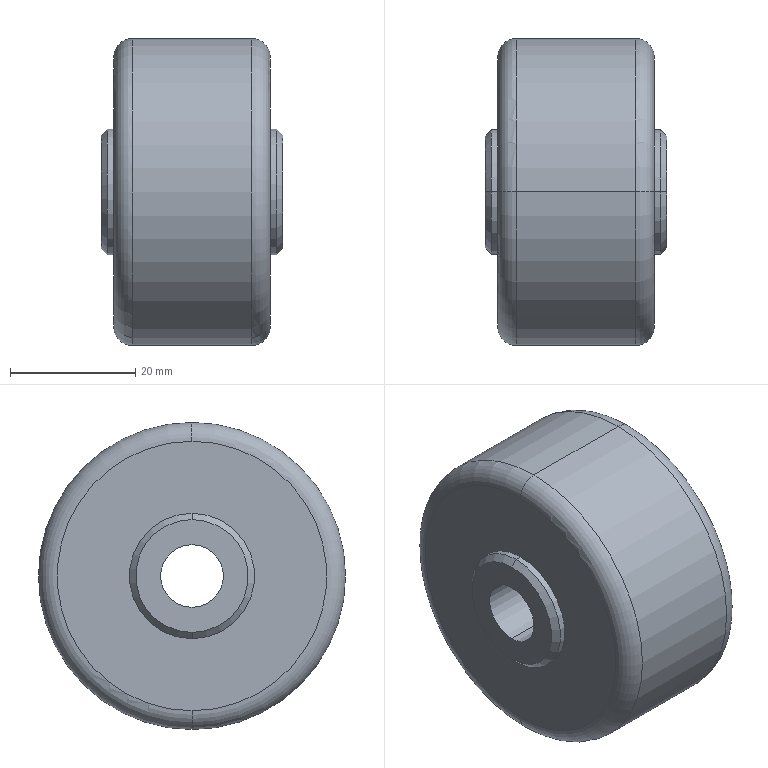Part | STEP file | _CGR51-60-U-001.stp | 1 solid | 20 faces | box 29 x 49 x 49 mm | volume 45483 mm3 | cylinder 8 | cone 4 | torus 4 | plane 4 | commonest cylinder face diameters 20 x4 10 x2 49 x2
STEP:
#1=CARTESIAN_POINT('',(-14.5,0.,-9.));
#2=VERTEX_POINT('',#1);
#3=CARTESIAN_POINT('',(-14.5,0.,9.));
#4=VERTEX_POINT('',#3);
#5=CARTESIAN_POINT('',(-14.5,0.,0.));
#6=DIRECTION('',(1.,0.,0.));
#7=DIRECTION('',(0.,0.,-1.));
#8=AXIS2_PLACEMENT_3D('',#5,#6,#7);
#9=CIRCLE('',#8,9.);
#10=EDGE_CURVE('',#2,#4,#9,.T.);
#11=ORIENTED_EDGE('',*,*,#10,.T.);
#12=CARTESIAN_POINT('',(-13.5,0.,10.));
#13=VERTEX_POINT('',#12);
#14=CARTESIAN_POINT('',(-13.5,0.,10.));
#15=DIRECTION('',(0.7071,0.,0.7071));
#16=VECTOR('',#15,1000.);
#17=LINE('',#14,#16);
#18=EDGE_CURVE('',#4,#13,#17,.T.);
#19=ORIENTED_EDGE('',*,*,#18,.T.);
#20=CARTESIAN_POINT('',(-13.5,0.,-10.));
#21=VERTEX_POINT('',#20);
#22=CARTESIAN_POINT('',(-13.5,0.,0.));
#23=DIRECTION('',(1.,0.,0.));
#24=DIRECTION('',(0.,0.,-1.));
#25=AXIS2_PLACEMENT_3D('',#22,#23,#24);
#26=CIRCLE('',#25,10.);
#27=EDGE_CURVE('',#21,#13,#26,.T.);
#28=ORIENTED_EDGE('',*,*,#27,.F.);
#29=CARTESIAN_POINT('',(-13.5,0.,-10.));
#30=DIRECTION('',(0.7071,0.,-0.7071));
#31=VECTOR('',#30,1000.);
#32=LINE('',#29,#31);
#33=EDGE_CURVE('',#2,#21,#32,.T.);
#34=ORIENTED_EDGE('',*,*,#33,.F.);
#35=EDGE_LOOP('',(#11,#19,#28,#34));
#36=FACE_OUTER_BOUND('',#35,.T.);
#37=CARTESIAN_POINT('',(-13.5,0.,0.));
#38=DIRECTION('',(1.,0.,0.));
#39=DIRECTION('',(0.,0.,-1.));
#40=AXIS2_PLACEMENT_3D('',#37,#38,#39);
#41=CONICAL_SURFACE('',#40,10.,0.7854);
#42=ADVANCED_FACE('',(#36),#41,.T.);
#43=CARTESIAN_POINT('',(14.5,0.,-5.));
#44=VERTEX_POINT('',#43);
#45=CARTESIAN_POINT('',(14.5,0.,5.));
#46=VERTEX_POINT('',#45);
#47=CARTESIAN_POINT('',(14.5,0.,0.));
#48=DIRECTION('',(1.,0.,0.));
#49=DIRECTION('',(0.,0.,-1.));
#50=AXIS2_PLACEMENT_3D('',#47,#48,#49);
#51=CIRCLE('',#50,5.);
#52=EDGE_CURVE('',#44,#46,#51,.T.);
#53=ORIENTED_EDGE('',*,*,#52,.T.);
#54=CARTESIAN_POINT('',(-14.5,0.,5.));
#55=VERTEX_POINT('',#54);
#56=CARTESIAN_POINT('',(50.,0.,5.));
#57=DIRECTION('',(-1.,0.,0.));
#58=VECTOR('',#57,1000.);
#59=LINE('',#56,#58);
#60=EDGE_CURVE('',#46,#55,#59,.T.);
#61=ORIENTED_EDGE('',*,*,#60,.T.);
#62=CARTESIAN_POINT('',(-14.5,0.,-5.));
#63=VERTEX_POINT('',#62);
#64=CARTESIAN_POINT('',(-14.5,0.,0.));
#65=DIRECTION('',(1.,0.,0.));
#66=DIRECTION('',(0.,0.,-1.));
#67=AXIS2_PLACEMENT_3D('',#64,#65,#66);
#68=CIRCLE('',#67,5.);
#69=EDGE_CURVE('',#63,#55,#68,.T.);
#70=ORIENTED_EDGE('',*,*,#69,.F.);
#71=CARTESIAN_POINT('',(50.,0.,-5.));
#72=DIRECTION('',(-1.,0.,0.));
#73=VECTOR('',#72,1000.);
#74=LINE('',#71,#73);
#75=EDGE_CURVE('',#44,#63,#74,.T.);
#76=ORIENTED_EDGE('',*,*,#75,.F.);
#77=EDGE_LOOP('',(#53,#61,#70,#76));
#78=FACE_OUTER_BOUND('',#77,.T.);
#79=CARTESIAN_POINT('',(50.,0.,0.));
#80=DIRECTION('',(-1.,0.,0.));
#81=DIRECTION('',(0.,0.,-1.));
#82=AXIS2_PLACEMENT_3D('',#79,#80,#81);
#83=CYLINDRICAL_SURFACE('',#82,5.);
#84=ADVANCED_FACE('',(#78),#83,.F.);
#85=CARTESIAN_POINT('',(14.5,0.,-9.));
#86=VERTEX_POINT('',#85);
#87=CARTESIAN_POINT('',(14.5,0.,9.));
#88=VERTEX_POINT('',#87);
#89=CARTESIAN_POINT('',(14.5,0.,0.));
#90=DIRECTION('',(1.,0.,0.));
#91=DIRECTION('',(0.,0.,-1.));
#92=AXIS2_PLACEMENT_3D('',#89,#90,#91);
#93=CIRCLE('',#92,9.);
#94=EDGE_CURVE('',#86,#88,#93,.T.);
#95=ORIENTED_EDGE('',*,*,#94,.F.);
#96=CARTESIAN_POINT('',(13.5,0.,-10.));
#97=VERTEX_POINT('',#96);
#98=CARTESIAN_POINT('',(14.5,0.,-9.));
#99=DIRECTION('',(-0.7071,0.,-0.7071));
#100=VECTOR('',#99,1000.);
#101=LINE('',#98,#100);
#102=EDGE_CURVE('',#86,#97,#101,.T.);
#103=ORIENTED_EDGE('',*,*,#102,.T.);
#104=CARTESIAN_POINT('',(13.5,0.,10.));
#105=VERTEX_POINT('',#104);
#106=CARTESIAN_POINT('',(13.5,0.,0.));
#107=DIRECTION('',(1.,0.,0.));
#108=DIRECTION('',(0.,0.,-1.));
#109=AXIS2_PLACEMENT_3D('',#106,#107,#108);
#110=CIRCLE('',#109,10.);
#111=EDGE_CURVE('',#97,#105,#110,.T.);
#112=ORIENTED_EDGE('',*,*,#111,.T.);
#113=CARTESIAN_POINT('',(14.5,0.,9.));
#114=DIRECTION('',(-0.7071,0.,0.7071));
#115=VECTOR('',#114,1000.);
#116=LINE('',#113,#115);
#117=EDGE_CURVE('',#88,#105,#116,.T.);
#118=ORIENTED_EDGE('',*,*,#117,.F.);
#119=EDGE_LOOP('',(#95,#103,#112,#118));
#120=FACE_OUTER_BOUND('',#119,.T.);
#121=CARTESIAN_POINT('',(14.5,0.,0.));
#122=DIRECTION('',(-1.,0.,0.));
#123=DIRECTION('',(0.,0.,1.));
#124=AXIS2_PLACEMENT_3D('',#121,#122,#123);
#125=CONICAL_SURFACE('',#124,9.,0.7854);
#126=ADVANCED_FACE('',(#120),#125,.T.);
#127=CARTESIAN_POINT('',(13.5,0.,0.));
#128=DIRECTION('',(1.,0.,0.));
#129=DIRECTION('',(0.,0.,-1.));
#130=AXIS2_PLACEMENT_3D('',#127,#128,#129);
#131=CIRCLE('',#130,10.);
#132=EDGE_CURVE('',#105,#97,#131,.T.);
#133=ORIENTED_EDGE('',*,*,#132,.F.);
#134=CARTESIAN_POINT('',(12.5,0.,10.));
#135=VERTEX_POINT('',#134);
#136=CARTESIAN_POINT('',(50.,0.,10.));
#137=DIRECTION('',(-1.,0.,0.));
#138=VECTOR('',#137,1000.);
#139=LINE('',#136,#138);
#140=EDGE_CURVE('',#105,#135,#139,.T.);
#141=ORIENTED_EDGE('',*,*,#140,.T.);
#142=CARTESIAN_POINT('',(12.5,0.,-10.));
#143=VERTEX_POINT('',#142);
#144=CARTESIAN_POINT('',(12.5,0.,0.));
#145=DIRECTION('',(1.,0.,0.));
#146=DIRECTION('',(0.,0.,-1.));
#147=AXIS2_PLACEMENT_3D('',#144,#145,#146);
#148=CIRCLE('',#147,10.);
#149=EDGE_CURVE('',#135,#143,#148,.T.);
#150=ORIENTED_EDGE('',*,*,#149,.T.);
#151=CARTESIAN_POINT('',(50.,0.,-10.));
#152=DIRECTION('',(-1.,0.,0.));
#153=VECTOR('',#152,1000.);
#154=LINE('',#151,#153);
#155=EDGE_CURVE('',#97,#143,#154,.T.);
#156=ORIENTED_EDGE('',*,*,#155,.F.);
#157=EDGE_LOOP('',(#133,#141,#150,#156));
#158=FACE_OUTER_BOUND('',#157,.T.);
#159=CARTESIAN_POINT('',(50.,0.,0.));
#160=DIRECTION('',(-1.,0.,0.));
#161=DIRECTION('',(0.,0.,-1.));
#162=AXIS2_PLACEMENT_3D('',#159,#160,#161);
#163=CYLINDRICAL_SURFACE('',#162,10.);
#164=ADVANCED_FACE('',(#158),#163,.T.);
#165=CARTESIAN_POINT('',(9.5,0.,-24.5));
#166=VERTEX_POINT('',#165);
#167=CARTESIAN_POINT('',(9.5,0.,24.5));
#168=VERTEX_POINT('',#167);
#169=CARTESIAN_POINT('',(9.5,0.,0.));
#170=DIRECTION('',(1.,0.,0.));
#171=DIRECTION('',(0.,0.,-1.));
#172=AXIS2_PLACEMENT_3D('',#169,#170,#171);
#173=CIRCLE('',#172,24.5);
#174=EDGE_CURVE('',#166,#168,#173,.T.);
#175=ORIENTED_EDGE('',*,*,#174,.T.);
#176=CARTESIAN_POINT('',(12.5,0.,21.5));
#177=VERTEX_POINT('',#176);
#178=CARTESIAN_POINT('',(9.5,0.,21.5));
#179=DIRECTION('',(0.,1.,0.));
#180=DIRECTION('',(0.,0.,1.));
#181=AXIS2_PLACEMENT_3D('',#178,#179,#180);
#182=CIRCLE('',#181,3.);
#183=EDGE_CURVE('',#168,#177,#182,.T.);
#184=ORIENTED_EDGE('',*,*,#183,.T.);
#185=CARTESIAN_POINT('',(12.5,0.,-21.5));
#186=VERTEX_POINT('',#185);
#187=CARTESIAN_POINT('',(12.5,0.,0.));
#188=DIRECTION('',(1.,0.,0.));
#189=DIRECTION('',(0.,0.,-1.));
#190=AXIS2_PLACEMENT_3D('',#187,#188,#189);
#191=CIRCLE('',#190,21.5);
#192=EDGE_CURVE('',#186,#177,#191,.T.);
#193=ORIENTED_EDGE('',*,*,#192,.F.);
#194=CARTESIAN_POINT('',(9.5,0.,-21.5));
#195=DIRECTION('',(0.,-1.,0.));
#196=DIRECTION('',(0.,0.,-1.));
#197=AXIS2_PLACEMENT_3D('',#194,#195,#196);
#198=CIRCLE('',#197,3.);
#199=EDGE_CURVE('',#166,#186,#198,.T.);
#200=ORIENTED_EDGE('',*,*,#199,.F.);
#201=EDGE_LOOP('',(#175,#184,#193,#200));
#202=FACE_OUTER_BOUND('',#201,.T.);
#203=CARTESIAN_POINT('',(9.5,0.,0.));
#204=DIRECTION('',(1.,0.,0.));
#205=DIRECTION('',(0.,0.,-1.));
#206=AXIS2_PLACEMENT_3D('',#203,#204,#205);
#207=TOROIDAL_SURFACE('',#206,21.5,3.);
#208=ADVANCED_FACE('',(#202),#207,.T.);
#209=CARTESIAN_POINT('',(9.5,0.,0.));
#210=DIRECTION('',(1.,0.,0.));
#211=DIRECTION('',(0.,0.,-1.));
#212=AXIS2_PLACEMENT_3D('',#209,#210,#211);
#213=CIRCLE('',#212,24.5);
#214=EDGE_CURVE('',#168,#166,#213,.T.);
#215=ORIENTED_EDGE('',*,*,#214,.F.);
#216=CARTESIAN_POINT('',(-9.5,0.,24.5));
#217=VERTEX_POINT('',#216);
#218=CARTESIAN_POINT('',(50.,0.,24.5));
#219=DIRECTION('',(-1.,0.,0.));
#220=VECTOR('',#219,1000.);
#221=LINE('',#218,#220);
#222=EDGE_CURVE('',#168,#217,#221,.T.);
#223=ORIENTED_EDGE('',*,*,#222,.T.);
#224=CARTESIAN_POINT('',(-9.5,0.,-24.5));
#225=VERTEX_POINT('',#224);
#226=CARTESIAN_POINT('',(-9.5,0.,0.));
#227=DIRECTION('',(1.,0.,0.));
#228=DIRECTION('',(0.,0.,-1.));
#229=AXIS2_PLACEMENT_3D('',#226,#227,#228);
#230=CIRCLE('',#229,24.5);
#231=EDGE_CURVE('',#217,#225,#230,.T.);
#232=ORIENTED_EDGE('',*,*,#231,.T.);
#233=CARTESIAN_POINT('',(50.,0.,-24.5));
#234=DIRECTION('',(-1.,0.,0.));
#235=VECTOR('',#234,1000.);
#236=LINE('',#233,#235);
#237=EDGE_CURVE('',#166,#225,#236,.T.);
#238=ORIENTED_EDGE('',*,*,#237,.F.);
#239=EDGE_LOOP('',(#215,#223,#232,#238));
#240=FACE_OUTER_BOUND('',#239,.T.);
#241=CARTESIAN_POINT('',(50.,0.,0.));
#242=DIRECTION('',(-1.,0.,0.));
#243=DIRECTION('',(0.,0.,-1.));
#244=AXIS2_PLACEMENT_3D('',#241,#242,#243);
#245=CYLINDRICAL_SURFACE('',#244,24.5);
#246=ADVANCED_FACE('',(#240),#245,.T.);
#247=CARTESIAN_POINT('',(-12.5,0.,-21.5));
#248=VERTEX_POINT('',#247);
#249=CARTESIAN_POINT('',(-12.5,0.,21.5));
#250=VERTEX_POINT('',#249);
#251=CARTESIAN_POINT('',(-12.5,0.,0.));
#252=DIRECTION('',(1.,0.,0.));
#253=DIRECTION('',(0.,0.,-1.));
#254=AXIS2_PLACEMENT_3D('',#251,#252,#253);
#255=CIRCLE('',#254,21.5);
#256=EDGE_CURVE('',#248,#250,#255,.T.);
#257=ORIENTED_EDGE('',*,*,#256,.T.);
#258=CARTESIAN_POINT('',(-9.5,0.,21.5));
#259=DIRECTION('',(0.,1.,0.));
#260=DIRECTION('',(0.,0.,1.));
#261=AXIS2_PLACEMENT_3D('',#258,#259,#260);
#262=CIRCLE('',#261,3.);
#263=EDGE_CURVE('',#250,#217,#262,.T.);
#264=ORIENTED_EDGE('',*,*,#263,.T.);
#265=CARTESIAN_POINT('',(-9.5,0.,0.));
#266=DIRECTION('',(1.,0.,0.));
#267=DIRECTION('',(0.,0.,-1.));
#268=AXIS2_PLACEMENT_3D('',#265,#266,#267);
#269=CIRCLE('',#268,24.5);
#270=EDGE_CURVE('',#225,#217,#269,.T.);
#271=ORIENTED_EDGE('',*,*,#270,.F.);
#272=CARTESIAN_POINT('',(-9.5,0.,-21.5));
#273=DIRECTION('',(0.,-1.,0.));
#274=DIRECTION('',(0.,0.,-1.));
#275=AXIS2_PLACEMENT_3D('',#272,#273,#274);
#276=CIRCLE('',#275,3.);
#277=EDGE_CURVE('',#248,#225,#276,.T.);
#278=ORIENTED_EDGE('',*,*,#277,.F.);
#279=EDGE_LOOP('',(#257,#264,#271,#278));
#280=FACE_OUTER_BOUND('',#279,.T.);
#281=CARTESIAN_POINT('',(-9.5,0.,0.));
#282=DIRECTION('',(1.,0.,0.));
#283=DIRECTION('',(0.,0.,-1.));
#284=AXIS2_PLACEMENT_3D('',#281,#282,#283);
#285=TOROIDAL_SURFACE('',#284,21.5,3.);
#286=ADVANCED_FACE('',(#280),#285,.T.);
#287=CARTESIAN_POINT('',(-12.5,0.,10.));
#288=VERTEX_POINT('',#287);
#289=CARTESIAN_POINT('',(-12.5,0.,-10.));
#290=VERTEX_POINT('',#289);
#291=CARTESIAN_POINT('',(-12.5,0.,0.));
#292=DIRECTION('',(1.,0.,0.));
#293=DIRECTION('',(0.,0.,-1.));
#294=AXIS2_PLACEMENT_3D('',#291,#292,#293);
#295=CIRCLE('',#294,10.);
#296=EDGE_CURVE('',#288,#290,#295,.T.);
#297=ORIENTED_EDGE('',*,*,#296,.F.);
#298=CARTESIAN_POINT('',(50.,0.,10.));
#299=DIRECTION('',(-1.,0.,0.));
#300=VECTOR('',#299,1000.);
#301=LINE('',#298,#300);
#302=EDGE_CURVE('',#288,#13,#301,.T.);
#303=ORIENTED_EDGE('',*,*,#302,.T.);
#304=CARTESIAN_POINT('',(-13.5,0.,0.));
#305=DIRECTION('',(1.,0.,0.));
#306=DIRECTION('',(0.,0.,-1.));
#307=AXIS2_PLACEMENT_3D('',#304,#305,#306);
#308=CIRCLE('',#307,10.);
#309=EDGE_CURVE('',#13,#21,#308,.T.);
#310=ORIENTED_EDGE('',*,*,#309,.T.);
#311=CARTESIAN_POINT('',(50.,0.,-10.));
#312=DIRECTION('',(-1.,0.,0.));
#313=VECTOR('',#312,1000.);
#314=LINE('',#311,#313);
#315=EDGE_CURVE('',#290,#21,#314,.T.);
#316=ORIENTED_EDGE('',*,*,#315,.F.);
#317=EDGE_LOOP('',(#297,#303,#310,#316));
#318=FACE_OUTER_BOUND('',#317,.T.);
#319=CARTESIAN_POINT('',(50.,0.,0.));
#320=DIRECTION('',(-1.,0.,0.));
#321=DIRECTION('',(0.,0.,-1.));
#322=AXIS2_PLACEMENT_3D('',#319,#320,#321);
#323=CYLINDRICAL_SURFACE('',#322,10.);
#324=ADVANCED_FACE('',(#318),#323,.T.);
#325=ORIENTED_EDGE('',*,*,#302,.F.);
#326=CARTESIAN_POINT('',(-12.5,0.,0.));
#327=DIRECTION('',(1.,0.,0.));
#328=DIRECTION('',(0.,0.,-1.));
#329=AXIS2_PLACEMENT_3D('',#326,#327,#328);
#330=CIRCLE('',#329,10.);
#331=EDGE_CURVE('',#290,#288,#330,.T.);
#332=ORIENTED_EDGE('',*,*,#331,.F.);
#333=ORIENTED_EDGE('',*,*,#315,.T.);
#334=ORIENTED_EDGE('',*,*,#27,.T.);
#335=EDGE_LOOP('',(#325,#332,#333,#334));
#336=FACE_OUTER_BOUND('',#335,.T.);
#337=CARTESIAN_POINT('',(50.,0.,0.));
#338=DIRECTION('',(-1.,0.,0.));
#339=DIRECTION('',(0.,0.,-1.));
#340=AXIS2_PLACEMENT_3D('',#337,#338,#339);
#341=CYLINDRICAL_SURFACE('',#340,10.);
#342=ADVANCED_FACE('',(#336),#341,.T.);
#343=ORIENTED_EDGE('',*,*,#331,.T.);
#344=ORIENTED_EDGE('',*,*,#296,.T.);
#345=EDGE_LOOP('',(#343,#344));
#346=FACE_BOUND('',#345,.T.);
#347=ORIENTED_EDGE('',*,*,#256,.F.);
#348=CARTESIAN_POINT('',(-12.5,0.,0.));
#349=DIRECTION('',(1.,0.,0.));
#350=DIRECTION('',(0.,0.,-1.));
#351=AXIS2_PLACEMENT_3D('',#348,#349,#350);
#352=CIRCLE('',#351,21.5);
#353=EDGE_CURVE('',#250,#248,#352,.T.);
#354=ORIENTED_EDGE('',*,*,#353,.F.);
#355=EDGE_LOOP('',(#347,#354));
#356=FACE_OUTER_BOUND('',#355,.T.);
#357=CARTESIAN_POINT('',(-12.5,21.5,0.));
#358=DIRECTION('',(-1.,0.,0.));
#359=DIRECTION('',(0.,0.,1.));
#360=AXIS2_PLACEMENT_3D('',#357,#358,#359);
#361=PLANE('',#360);
#362=ADVANCED_FACE('',(#346,#356),#361,.T.);
#363=ORIENTED_EDGE('',*,*,#263,.F.);
#364=ORIENTED_EDGE('',*,*,#353,.T.);
#365=ORIENTED_EDGE('',*,*,#277,.T.);
#366=ORIENTED_EDGE('',*,*,#231,.F.);
#367=EDGE_LOOP('',(#363,#364,#365,#366));
#368=FACE_OUTER_BOUND('',#367,.T.);
#369=CARTESIAN_POINT('',(-9.5,0.,0.));
#370=DIRECTION('',(1.,0.,0.));
#371=DIRECTION('',(0.,0.,-1.));
#372=AXIS2_PLACEMENT_3D('',#369,#370,#371);
#373=TOROIDAL_SURFACE('',#372,21.5,3.);
#374=ADVANCED_FACE('',(#368),#373,.T.);
#375=ORIENTED_EDGE('',*,*,#222,.F.);
#376=ORIENTED_EDGE('',*,*,#174,.F.);
#377=ORIENTED_EDGE('',*,*,#237,.T.);
#378=ORIENTED_EDGE('',*,*,#270,.T.);
#379=EDGE_LOOP('',(#375,#376,#377,#378));
#380=FACE_OUTER_BOUND('',#379,.T.);
#381=CARTESIAN_POINT('',(50.,0.,0.));
#382=DIRECTION('',(-1.,0.,0.));
#383=DIRECTION('',(0.,0.,-1.));
#384=AXIS2_PLACEMENT_3D('',#381,#382,#383);
#385=CYLINDRICAL_SURFACE('',#384,24.5);
#386=ADVANCED_FACE('',(#380),#385,.T.);
#387=ORIENTED_EDGE('',*,*,#183,.F.);
#388=ORIENTED_EDGE('',*,*,#214,.T.);
#389=ORIENTED_EDGE('',*,*,#199,.T.);
#390=CARTESIAN_POINT('',(12.5,0.,0.));
#391=DIRECTION('',(1.,0.,0.));
#392=DIRECTION('',(0.,0.,-1.));
#393=AXIS2_PLACEMENT_3D('',#390,#391,#392);
#394=CIRCLE('',#393,21.5);
#395=EDGE_CURVE('',#177,#186,#394,.T.);
#396=ORIENTED_EDGE('',*,*,#395,.F.);
#397=EDGE_LOOP('',(#387,#388,#389,#396));
#398=FACE_OUTER_BOUND('',#397,.T.);
#399=CARTESIAN_POINT('',(9.5,0.,0.));
#400=DIRECTION('',(1.,0.,0.));
#401=DIRECTION('',(0.,0.,-1.));
#402=AXIS2_PLACEMENT_3D('',#399,#400,#401);
#403=TOROIDAL_SURFACE('',#402,21.5,3.);
#404=ADVANCED_FACE('',(#398),#403,.T.);
#405=CARTESIAN_POINT('',(12.5,0.,0.));
#406=DIRECTION('',(1.,0.,0.));
#407=DIRECTION('',(0.,0.,-1.));
#408=AXIS2_PLACEMENT_3D('',#405,#406,#407);
#409=CIRCLE('',#408,10.);
#410=EDGE_CURVE('',#143,#135,#409,.T.);
#411=ORIENTED_EDGE('',*,*,#410,.F.);
#412=ORIENTED_EDGE('',*,*,#149,.F.);
#413=EDGE_LOOP('',(#411,#412));
#414=FACE_BOUND('',#413,.T.);
#415=ORIENTED_EDGE('',*,*,#192,.T.);
#416=ORIENTED_EDGE('',*,*,#395,.T.);
#417=EDGE_LOOP('',(#415,#416));
#418=FACE_OUTER_BOUND('',#417,.T.);
#419=CARTESIAN_POINT('',(12.5,10.,0.));
#420=DIRECTION('',(1.,0.,0.));
#421=DIRECTION('',(0.,1.,0.));
#422=AXIS2_PLACEMENT_3D('',#419,#420,#421);
#423=PLANE('',#422);
#424=ADVANCED_FACE('',(#414,#418),#423,.T.);
#425=ORIENTED_EDGE('',*,*,#140,.F.);
#426=ORIENTED_EDGE('',*,*,#111,.F.);
#427=ORIENTED_EDGE('',*,*,#155,.T.);
#428=ORIENTED_EDGE('',*,*,#410,.T.);
#429=EDGE_LOOP('',(#425,#426,#427,#428));
#430=FACE_OUTER_BOUND('',#429,.T.);
#431=CARTESIAN_POINT('',(50.,0.,0.));
#432=DIRECTION('',(-1.,0.,0.));
#433=DIRECTION('',(0.,0.,-1.));
#434=AXIS2_PLACEMENT_3D('',#431,#432,#433);
#435=CYLINDRICAL_SURFACE('',#434,10.);
#436=ADVANCED_FACE('',(#430),#435,.T.);
#437=ORIENTED_EDGE('',*,*,#102,.F.);
#438=CARTESIAN_POINT('',(14.5,0.,0.));
#439=DIRECTION('',(1.,0.,0.));
#440=DIRECTION('',(0.,0.,-1.));
#441=AXIS2_PLACEMENT_3D('',#438,#439,#440);
#442=CIRCLE('',#441,9.);
#443=EDGE_CURVE('',#88,#86,#442,.T.);
#444=ORIENTED_EDGE('',*,*,#443,.F.);
#445=ORIENTED_EDGE('',*,*,#117,.T.);
#446=ORIENTED_EDGE('',*,*,#132,.T.);
#447=EDGE_LOOP('',(#437,#444,#445,#446));
#448=FACE_OUTER_BOUND('',#447,.T.);
#449=CARTESIAN_POINT('',(14.5,0.,0.));
#450=DIRECTION('',(-1.,0.,0.));
#451=DIRECTION('',(0.,0.,1.));
#452=AXIS2_PLACEMENT_3D('',#449,#450,#451);
#453=CONICAL_SURFACE('',#452,9.,0.7854);
#454=ADVANCED_FACE('',(#448),#453,.T.);
#455=ORIENTED_EDGE('',*,*,#52,.F.);
#456=CARTESIAN_POINT('',(14.5,0.,0.));
#457=DIRECTION('',(1.,0.,0.));
#458=DIRECTION('',(0.,0.,-1.));
#459=AXIS2_PLACEMENT_3D('',#456,#457,#458);
#460=CIRCLE('',#459,5.);
#461=EDGE_CURVE('',#46,#44,#460,.T.);
#462=ORIENTED_EDGE('',*,*,#461,.F.);
#463=EDGE_LOOP('',(#455,#462));
#464=FACE_BOUND('',#463,.T.);
#465=ORIENTED_EDGE('',*,*,#443,.T.);
#466=ORIENTED_EDGE('',*,*,#94,.T.);
#467=EDGE_LOOP('',(#465,#466));
#468=FACE_OUTER_BOUND('',#467,.T.);
#469=CARTESIAN_POINT('',(14.5,5.,0.));
#470=DIRECTION('',(1.,0.,0.));
#471=DIRECTION('',(0.,1.,0.));
#472=AXIS2_PLACEMENT_3D('',#469,#470,#471);
#473=PLANE('',#472);
#474=ADVANCED_FACE('',(#464,#468),#473,.T.);
#475=ORIENTED_EDGE('',*,*,#60,.F.);
#476=ORIENTED_EDGE('',*,*,#461,.T.);
#477=ORIENTED_EDGE('',*,*,#75,.T.);
#478=CARTESIAN_POINT('',(-14.5,0.,0.));
#479=DIRECTION('',(1.,0.,0.));
#480=DIRECTION('',(0.,0.,-1.));
#481=AXIS2_PLACEMENT_3D('',#478,#479,#480);
#482=CIRCLE('',#481,5.);
#483=EDGE_CURVE('',#55,#63,#482,.T.);
#484=ORIENTED_EDGE('',*,*,#483,.F.);
#485=EDGE_LOOP('',(#475,#476,#477,#484));
#486=FACE_OUTER_BOUND('',#485,.T.);
#487=CARTESIAN_POINT('',(50.,0.,0.));
#488=DIRECTION('',(-1.,0.,0.));
#489=DIRECTION('',(0.,0.,-1.));
#490=AXIS2_PLACEMENT_3D('',#487,#488,#489);
#491=CYLINDRICAL_SURFACE('',#490,5.);
#492=ADVANCED_FACE('',(#486),#491,.F.);
#493=ORIENTED_EDGE('',*,*,#69,.T.);
#494=ORIENTED_EDGE('',*,*,#483,.T.);
#495=EDGE_LOOP('',(#493,#494));
#496=FACE_BOUND('',#495,.T.);
#497=ORIENTED_EDGE('',*,*,#10,.F.);
#498=CARTESIAN_POINT('',(-14.5,0.,0.));
#499=DIRECTION('',(1.,0.,0.));
#500=DIRECTION('',(0.,0.,-1.));
#501=AXIS2_PLACEMENT_3D('',#498,#499,#500);
#502=CIRCLE('',#501,9.);
#503=EDGE_CURVE('',#4,#2,#502,.T.);
#504=ORIENTED_EDGE('',*,*,#503,.F.);
#505=EDGE_LOOP('',(#497,#504));
#506=FACE_OUTER_BOUND('',#505,.T.);
#507=CARTESIAN_POINT('',(-14.5,9.,0.));
#508=DIRECTION('',(-1.,0.,0.));
#509=DIRECTION('',(0.,0.,1.));
#510=AXIS2_PLACEMENT_3D('',#507,#508,#509);
#511=PLANE('',#510);
#512=ADVANCED_FACE('',(#496,#506),#511,.T.);
#513=ORIENTED_EDGE('',*,*,#18,.F.);
#514=ORIENTED_EDGE('',*,*,#503,.T.);
#515=ORIENTED_EDGE('',*,*,#33,.T.);
#516=ORIENTED_EDGE('',*,*,#309,.F.);
#517=EDGE_LOOP('',(#513,#514,#515,#516));
#518=FACE_OUTER_BOUND('',#517,.T.);
#519=CARTESIAN_POINT('',(-13.5,0.,0.));
#520=DIRECTION('',(1.,0.,0.));
#521=DIRECTION('',(0.,0.,-1.));
#522=AXIS2_PLACEMENT_3D('',#519,#520,#521);
#523=CONICAL_SURFACE('',#522,10.,0.7854);
#524=ADVANCED_FACE('',(#518),#523,.T.);
#525=CLOSED_SHELL('',(#42,#84,#126,#164,#208,#246,#286,#324,#342,#362,#374,#386,#404,#424,#436,#454,#474,#492,#512,#524));
#526=MANIFOLD_SOLID_BREP('',#525);
#527=CARTESIAN_POINT('',(0.,0.,0.));
#528=DIRECTION('',(0.,0.,1.));
#529=DIRECTION('',(1.,0.,0.));
#530=AXIS2_PLACEMENT_3D('',#527,#528,#529);
#531=(LENGTH_UNIT()NAMED_UNIT(*)SI_UNIT(.MILLI.,.METRE.));
#532=UNCERTAINTY_MEASURE_WITH_UNIT(LENGTH_MEASURE(0.00001),#531,'','');
#533=(NAMED_UNIT(*)PLANE_ANGLE_UNIT()SI_UNIT($,.RADIAN.));
#534=(NAMED_UNIT(*)SI_UNIT($,.STERADIAN.)SOLID_ANGLE_UNIT());
#535=(GEOMETRIC_REPRESENTATION_CONTEXT(3)GLOBAL_UNCERTAINTY_ASSIGNED_CONTEXT((#532))GLOBAL_UNIT_ASSIGNED_CONTEXT((#531,#533,#534))REPRESENTATION_CONTEXT('',''));
#536=ADVANCED_BREP_SHAPE_REPRESENTATION('',(#526,#530),#535);